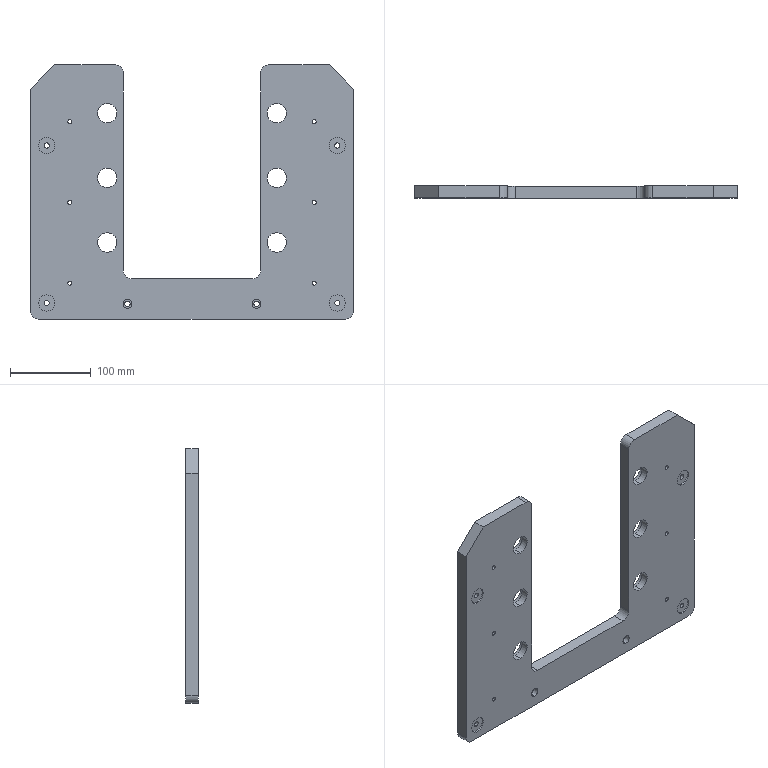Part | STEP file | PN_0003 | 1 solid | 108 faces | box 400 x 15 x 315 mm | volume 1138040 mm3 | cylinder 78 | plane 30 | commonest cylinder face diameters 5 x12 6.6 x12 11 x12 24.05 x12 31.1 x12 20.2 x8